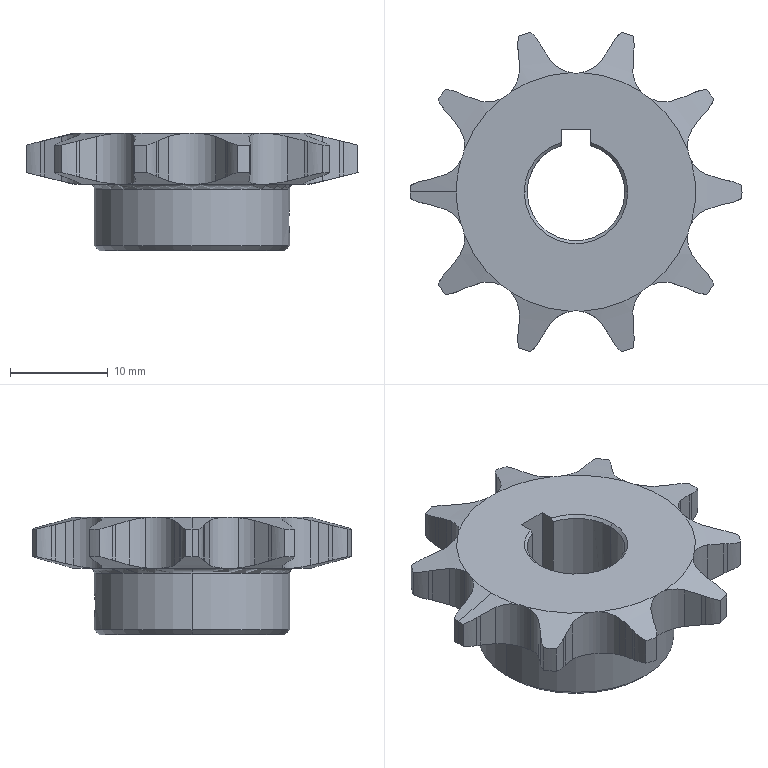Part | STEP file | BZJ-LSX-RGX 主动链轮06B-10齿_内Holeφ10 | 1 solid | 134 faces | box 34 x 32.715 x 12 mm | volume 4151 mm3 | cylinder 76 | cone 30 | plane 26 | torus 2 | commonest cylinder face diameters 9.51 x22 16.642 x22 6.482 x12 34 x11 2.5 x4 10 x3